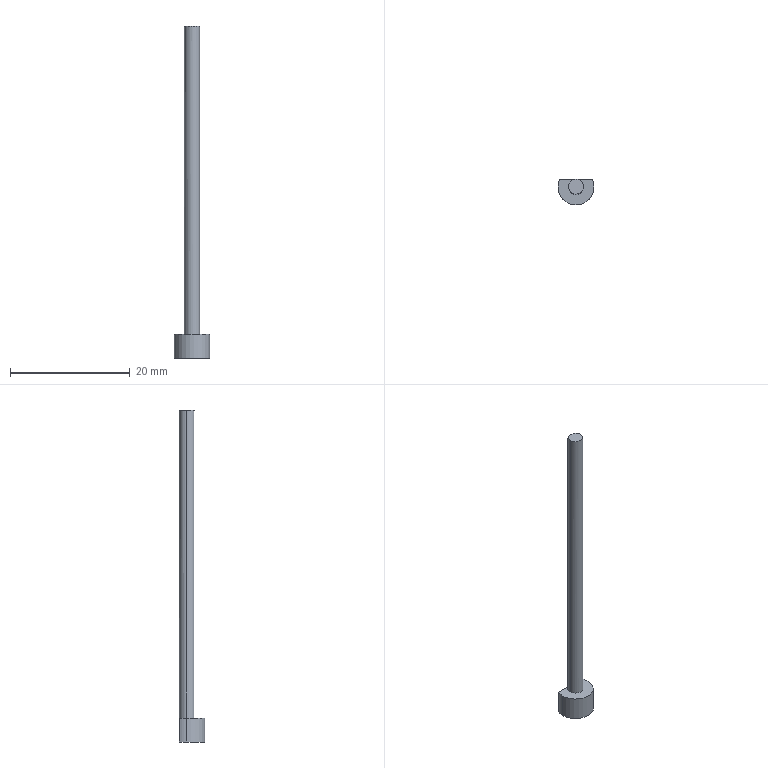Part | STEP file | 1 solid | 10 faces | box 6 x 4.256 x 55.458 mm | volume 340.576 mm3 | cylinder 5 | plane 5 | commonest cylinder face diameters 6 x3 2.513 x2
STEP:
#1=CARTESIAN_POINT('',(0.,0.,0.));
#2=DIRECTION('',(0.,0.,1.));
#3=DIRECTION('',(1.,0.,0.));
#4=AXIS2_PLACEMENT_3D('',#1,#2,#3);
#5=CARTESIAN_POINT('',(-20.312,64.873,-51.47));
#6=VERTEX_POINT('',#5);
#7=CARTESIAN_POINT('',(-20.587,63.617,-51.47));
#8=VERTEX_POINT('',#7);
#9=CARTESIAN_POINT('',(-17.587,63.617,-51.47));
#10=DIRECTION('',(0.,0.,1.));
#11=DIRECTION('',(1.,0.,0.));
#12=AXIS2_PLACEMENT_3D('',#9,#10,#11);
#13=CIRCLE('',#12,3.);
#14=CARTESIAN_POINT('',(-17.587,63.617,-51.47));
#15=DIRECTION('',(0.,0.,1.));
#16=DIRECTION('',(1.,0.,0.));
#17=AXIS2_PLACEMENT_3D('',#14,#15,#16);
#18=CYLINDRICAL_SURFACE('',#17,3.);
#19=CARTESIAN_POINT('',(0.,0.));
#20=DIRECTION('',(1.,0.));
#21=VECTOR('',#20,1.);
#22=LINE('',#19,#21);
#23=(GEOMETRIC_REPRESENTATION_CONTEXT(2)PARAMETRIC_REPRESENTATION_CONTEXT()REPRESENTATION_CONTEXT('',''));
#24=DEFINITIONAL_REPRESENTATION('',(#22),#23);
#25=PCURVE('',#18,#24);
#26=CARTESIAN_POINT('',(-42.862,64.,-51.47));
#27=DIRECTION('',(0.,0.,1.));
#28=DIRECTION('',(1.,0.,0.));
#29=AXIS2_PLACEMENT_3D('',#26,#27,#28);
#30=PLANE('',#29);
#31=CARTESIAN_POINT('',(25.275,-0.3835));
#32=DIRECTION('',(1.,0.));
#33=AXIS2_PLACEMENT_2D('',#31,#32);
#34=CIRCLE('',#33,3.);
#35=(GEOMETRIC_REPRESENTATION_CONTEXT(2)PARAMETRIC_REPRESENTATION_CONTEXT()REPRESENTATION_CONTEXT('',''));
#36=DEFINITIONAL_REPRESENTATION('',(#34),#35);
#37=PCURVE('',#30,#36);
#38=SURFACE_CURVE('',#13,(#25,#37),.PCURVE_S1.);
#39=EDGE_CURVE('',#6,#8,#38,.T.);
#40=ORIENTED_EDGE('',*,*,#39,.T.);
#41=CARTESIAN_POINT('',(-20.587,63.617,-47.47));
#42=VERTEX_POINT('',#41);
#43=CARTESIAN_POINT('',(-20.587,63.617,-51.47));
#44=DIRECTION('',(0.,0.,1.));
#45=VECTOR('',#44,1.);
#46=LINE('',#43,#45);
#47=CARTESIAN_POINT('',(3.142,0.));
#48=DIRECTION('',(0.,1.));
#49=VECTOR('',#48,1.);
#50=LINE('',#47,#49);
#51=(GEOMETRIC_REPRESENTATION_CONTEXT(2)PARAMETRIC_REPRESENTATION_CONTEXT()REPRESENTATION_CONTEXT('',''));
#52=DEFINITIONAL_REPRESENTATION('',(#50),#51);
#53=PCURVE('',#18,#52);
#54=CARTESIAN_POINT('',(-17.587,63.617,-51.47));
#55=DIRECTION('',(0.,0.,1.));
#56=DIRECTION('',(1.,0.,0.));
#57=AXIS2_PLACEMENT_3D('',#54,#55,#56);
#58=CYLINDRICAL_SURFACE('',#57,3.);
#59=CARTESIAN_POINT('',(3.142,0.));
#60=DIRECTION('',(0.,1.));
#61=VECTOR('',#60,1.);
#62=LINE('',#59,#61);
#63=(GEOMETRIC_REPRESENTATION_CONTEXT(2)PARAMETRIC_REPRESENTATION_CONTEXT()REPRESENTATION_CONTEXT('',''));
#64=DEFINITIONAL_REPRESENTATION('',(#62),#63);
#65=PCURVE('',#58,#64);
#66=SURFACE_CURVE('',#46,(#53,#65),.PCURVE_S1.);
#67=EDGE_CURVE('',#8,#42,#66,.T.);
#68=ORIENTED_EDGE('',*,*,#67,.T.);
#69=CARTESIAN_POINT('',(-20.312,64.873,-47.47));
#70=VERTEX_POINT('',#69);
#71=CARTESIAN_POINT('',(-17.587,63.617,-47.47));
#72=DIRECTION('',(0.,0.,-1.));
#73=DIRECTION('',(-1.,0.,0.));
#74=AXIS2_PLACEMENT_3D('',#71,#72,#73);
#75=CIRCLE('',#74,3.);
#76=CARTESIAN_POINT('',(3.142,4.));
#77=DIRECTION('',(-1.,0.));
#78=VECTOR('',#77,1.);
#79=LINE('',#76,#78);
#80=(GEOMETRIC_REPRESENTATION_CONTEXT(2)PARAMETRIC_REPRESENTATION_CONTEXT()REPRESENTATION_CONTEXT('',''));
#81=DEFINITIONAL_REPRESENTATION('',(#79),#80);
#82=PCURVE('',#18,#81);
#83=CARTESIAN_POINT('',(-17.587,63.617,-47.47));
#84=DIRECTION('',(0.,0.,1.));
#85=DIRECTION('',(1.,0.,0.));
#86=AXIS2_PLACEMENT_3D('',#83,#84,#85);
#87=PLANE('',#86);
#88=CARTESIAN_POINT('',(-3.,0.));
#89=CARTESIAN_POINT('',(-3.,5.196));
#90=CARTESIAN_POINT('',(1.5,2.598));
#91=CARTESIAN_POINT('',(6.,0.));
#92=CARTESIAN_POINT('',(1.5,-2.598));
#93=CARTESIAN_POINT('',(-3.,-5.196));
#94=CARTESIAN_POINT('',(-3.,0.));
#95=(BOUNDED_CURVE()B_SPLINE_CURVE(2,(#88,#89,#90,#91,#92,#93,#94),.UNSPECIFIED.,.T.,.F.)B_SPLINE_CURVE_WITH_KNOTS((1,2,2,2,2,1),(-2.094,0.,2.094,4.189,6.283,8.378),.UNSPECIFIED.)CURVE()GEOMETRIC_REPRESENTATION_ITEM()RATIONAL_B_SPLINE_CURVE((1.,0.5,1.,0.5,1.,0.5,1.))REPRESENTATION_ITEM(''));
#96=(GEOMETRIC_REPRESENTATION_CONTEXT(2)PARAMETRIC_REPRESENTATION_CONTEXT()REPRESENTATION_CONTEXT('',''));
#97=DEFINITIONAL_REPRESENTATION('',(#95),#96);
#98=PCURVE('',#87,#97);
#99=SURFACE_CURVE('',#75,(#82,#98),.PCURVE_S1.);
#100=EDGE_CURVE('',#42,#70,#99,.T.);
#101=ORIENTED_EDGE('',*,*,#100,.T.);
#102=CARTESIAN_POINT('',(-20.312,64.873,-51.47));
#103=DIRECTION('',(0.,0.,-1.));
#104=VECTOR('',#103,1.);
#105=LINE('',#102,#104);
#106=CARTESIAN_POINT('',(2.71,0.));
#107=DIRECTION('',(0.,-1.));
#108=VECTOR('',#107,1.);
#109=LINE('',#106,#108);
#110=(GEOMETRIC_REPRESENTATION_CONTEXT(2)PARAMETRIC_REPRESENTATION_CONTEXT()REPRESENTATION_CONTEXT('',''));
#111=DEFINITIONAL_REPRESENTATION('',(#109),#110);
#112=PCURVE('',#18,#111);
#113=CARTESIAN_POINT('',(-17.587,64.873,-51.47));
#114=DIRECTION('',(0.,1.,0.));
#115=DIRECTION('',(0.,0.,1.));
#116=AXIS2_PLACEMENT_3D('',#113,#114,#115);
#117=PLANE('',#116);
#118=CARTESIAN_POINT('',(0.,-2.724));
#119=DIRECTION('',(-1.,0.));
#120=VECTOR('',#119,1.);
#121=LINE('',#118,#120);
#122=(GEOMETRIC_REPRESENTATION_CONTEXT(2)PARAMETRIC_REPRESENTATION_CONTEXT()REPRESENTATION_CONTEXT('',''));
#123=DEFINITIONAL_REPRESENTATION('',(#121),#122);
#124=PCURVE('',#117,#123);
#125=SURFACE_CURVE('',#105,(#112,#124),.PCURVE_S1.);
#126=EDGE_CURVE('',#70,#6,#125,.T.);
#127=ORIENTED_EDGE('',*,*,#126,.T.);
#128=EDGE_LOOP('',(#40,#68,#101,#127));
#129=FACE_BOUND('',#128,.T.);
#130=ADVANCED_FACE('',(#129),#18,.T.);
#131=ORIENTED_EDGE('',*,*,#67,.F.);
#132=CARTESIAN_POINT('',(-14.588,63.617,-51.47));
#133=VERTEX_POINT('',#132);
#134=CARTESIAN_POINT('',(-17.587,63.617,-51.47));
#135=DIRECTION('',(0.,0.,1.));
#136=DIRECTION('',(1.,0.,0.));
#137=AXIS2_PLACEMENT_3D('',#134,#135,#136);
#138=CIRCLE('',#137,3.);
#139=CARTESIAN_POINT('',(0.,0.));
#140=DIRECTION('',(1.,0.));
#141=VECTOR('',#140,1.);
#142=LINE('',#139,#141);
#143=(GEOMETRIC_REPRESENTATION_CONTEXT(2)PARAMETRIC_REPRESENTATION_CONTEXT()REPRESENTATION_CONTEXT('',''));
#144=DEFINITIONAL_REPRESENTATION('',(#142),#143);
#145=PCURVE('',#58,#144);
#146=CARTESIAN_POINT('',(25.275,-0.3835));
#147=DIRECTION('',(1.,0.));
#148=AXIS2_PLACEMENT_2D('',#146,#147);
#149=CIRCLE('',#148,3.);
#150=(GEOMETRIC_REPRESENTATION_CONTEXT(2)PARAMETRIC_REPRESENTATION_CONTEXT()REPRESENTATION_CONTEXT('',''));
#151=DEFINITIONAL_REPRESENTATION('',(#149),#150);
#152=PCURVE('',#30,#151);
#153=SURFACE_CURVE('',#138,(#145,#152),.PCURVE_S1.);
#154=EDGE_CURVE('',#8,#133,#153,.T.);
#155=ORIENTED_EDGE('',*,*,#154,.T.);
#156=CARTESIAN_POINT('',(-14.588,63.617,-47.47));
#157=VERTEX_POINT('',#156);
#158=CARTESIAN_POINT('',(-14.588,63.617,-51.47));
#159=DIRECTION('',(0.,0.,1.));
#160=VECTOR('',#159,1.);
#161=LINE('',#158,#160);
#162=CARTESIAN_POINT('',(6.283,0.));
#163=DIRECTION('',(0.,1.));
#164=VECTOR('',#163,1.);
#165=LINE('',#162,#164);
#166=(GEOMETRIC_REPRESENTATION_CONTEXT(2)PARAMETRIC_REPRESENTATION_CONTEXT()REPRESENTATION_CONTEXT('',''));
#167=DEFINITIONAL_REPRESENTATION('',(#165),#166);
#168=PCURVE('',#58,#167);
#169=CARTESIAN_POINT('',(-17.587,63.617,-51.47));
#170=DIRECTION('',(0.,0.,1.));
#171=DIRECTION('',(1.,0.,0.));
#172=AXIS2_PLACEMENT_3D('',#169,#170,#171);
#173=CYLINDRICAL_SURFACE('',#172,3.);
#174=CARTESIAN_POINT('',(0.,0.));
#175=DIRECTION('',(0.,1.));
#176=VECTOR('',#175,1.);
#177=LINE('',#174,#176);
#178=(GEOMETRIC_REPRESENTATION_CONTEXT(2)PARAMETRIC_REPRESENTATION_CONTEXT()REPRESENTATION_CONTEXT('',''));
#179=DEFINITIONAL_REPRESENTATION('',(#177),#178);
#180=PCURVE('',#173,#179);
#181=SURFACE_CURVE('',#161,(#168,#180),.PCURVE_S1.);
#182=EDGE_CURVE('',#133,#157,#181,.T.);
#183=ORIENTED_EDGE('',*,*,#182,.T.);
#184=CARTESIAN_POINT('',(-17.587,63.617,-47.47));
#185=DIRECTION('',(0.,0.,-1.));
#186=DIRECTION('',(-1.,0.,0.));
#187=AXIS2_PLACEMENT_3D('',#184,#185,#186);
#188=CIRCLE('',#187,3.);
#189=CARTESIAN_POINT('',(9.425,4.));
#190=DIRECTION('',(-1.,0.));
#191=VECTOR('',#190,1.);
#192=LINE('',#189,#191);
#193=(GEOMETRIC_REPRESENTATION_CONTEXT(2)PARAMETRIC_REPRESENTATION_CONTEXT()REPRESENTATION_CONTEXT('',''));
#194=DEFINITIONAL_REPRESENTATION('',(#192),#193);
#195=PCURVE('',#58,#194);
#196=CARTESIAN_POINT('',(-3.,0.));
#197=CARTESIAN_POINT('',(-3.,5.196));
#198=CARTESIAN_POINT('',(1.5,2.598));
#199=CARTESIAN_POINT('',(6.,0.));
#200=CARTESIAN_POINT('',(1.5,-2.598));
#201=CARTESIAN_POINT('',(-3.,-5.196));
#202=CARTESIAN_POINT('',(-3.,0.));
#203=(BOUNDED_CURVE()B_SPLINE_CURVE(2,(#196,#197,#198,#199,#200,#201,#202),.UNSPECIFIED.,.T.,.F.)B_SPLINE_CURVE_WITH_KNOTS((1,2,2,2,2,1),(-2.094,0.,2.094,4.189,6.283,8.378),.UNSPECIFIED.)CURVE()GEOMETRIC_REPRESENTATION_ITEM()RATIONAL_B_SPLINE_CURVE((1.,0.5,1.,0.5,1.,0.5,1.))REPRESENTATION_ITEM(''));
#204=(GEOMETRIC_REPRESENTATION_CONTEXT(2)PARAMETRIC_REPRESENTATION_CONTEXT()REPRESENTATION_CONTEXT('',''));
#205=DEFINITIONAL_REPRESENTATION('',(#203),#204);
#206=PCURVE('',#87,#205);
#207=SURFACE_CURVE('',#188,(#195,#206),.PCURVE_S1.);
#208=EDGE_CURVE('',#157,#42,#207,.T.);
#209=ORIENTED_EDGE('',*,*,#208,.T.);
#210=EDGE_LOOP('',(#131,#155,#183,#209));
#211=FACE_BOUND('',#210,.T.);
#212=ADVANCED_FACE('',(#211),#58,.T.);
#213=CARTESIAN_POINT('',(-18.844,63.617,3.922));
#214=VERTEX_POINT('',#213);
#215=CARTESIAN_POINT('',(-16.331,63.617,3.922));
#216=VERTEX_POINT('',#215);
#217=CARTESIAN_POINT('',(-18.844,63.617,3.922));
#218=CARTESIAN_POINT('',(-18.844,66.129,3.791));
#219=CARTESIAN_POINT('',(-16.331,66.129,3.791));
#220=CARTESIAN_POINT('',(-16.331,63.617,3.922));
#221=(BOUNDED_CURVE()B_SPLINE_CURVE(3,(#217,#218,#219,#220),.UNSPECIFIED.,.F.,.F.)B_SPLINE_CURVE_WITH_KNOTS((4,4),(4.712,7.854),.PIECEWISE_BEZIER_KNOTS.)CURVE()GEOMETRIC_REPRESENTATION_ITEM()RATIONAL_B_SPLINE_CURVE((1.,0.3333,0.3333,1.))REPRESENTATION_ITEM(''));
#222=CARTESIAN_POINT('',(-17.587,63.617,7.478));
#223=DIRECTION('',(0.,0.,-1.));
#224=DIRECTION('',(-1.,0.,0.));
#225=AXIS2_PLACEMENT_3D('',#222,#223,#224);
#226=CYLINDRICAL_SURFACE('',#225,1.256);
#227=CARTESIAN_POINT('',(0.,3.556));
#228=CARTESIAN_POINT('',(0.0303,3.558));
#229=CARTESIAN_POINT('',(0.09367,3.562));
#230=CARTESIAN_POINT('',(0.1977,3.569));
#231=CARTESIAN_POINT('',(0.3115,3.576));
#232=CARTESIAN_POINT('',(0.4356,3.584));
#233=CARTESIAN_POINT('',(0.5703,3.591));
#234=CARTESIAN_POINT('',(0.7158,3.599));
#235=CARTESIAN_POINT('',(0.8717,3.606));
#236=CARTESIAN_POINT('',(1.037,3.613));
#237=CARTESIAN_POINT('',(1.21,3.618));
#238=CARTESIAN_POINT('',(1.389,3.621));
#239=CARTESIAN_POINT('',(1.571,3.622));
#240=CARTESIAN_POINT('',(1.753,3.621));
#241=CARTESIAN_POINT('',(1.931,3.618));
#242=CARTESIAN_POINT('',(2.105,3.613));
#243=CARTESIAN_POINT('',(2.27,3.606));
#244=CARTESIAN_POINT('',(2.426,3.599));
#245=CARTESIAN_POINT('',(2.571,3.591));
#246=CARTESIAN_POINT('',(2.706,3.584));
#247=CARTESIAN_POINT('',(2.83,3.576));
#248=CARTESIAN_POINT('',(2.944,3.569));
#249=CARTESIAN_POINT('',(3.048,3.562));
#250=CARTESIAN_POINT('',(3.111,3.558));
#251=CARTESIAN_POINT('',(3.142,3.556));
#252=B_SPLINE_CURVE_WITH_KNOTS('',3,(#227,#228,#229,#230,#231,#232,#233,#234,#235,#236,#237,#238,#239,#240,#241,#242,#243,#244,#245,#246,#247,#248,#249,#250,#251),.UNSPECIFIED.,.F.,.F.,(4,1,1,1,1,1,1,1,1,1,1,1,1,1,1,1,1,1,1,1,1,1,4),(4.712,4.855,4.998,5.141,5.284,5.426,5.569,5.712,5.855,5.998,6.14,6.283,6.426,6.569,6.712,6.854,6.997,7.14,7.283,7.426,7.568,7.711,7.854),.QUASI_UNIFORM_KNOTS.);
#253=(GEOMETRIC_REPRESENTATION_CONTEXT(2)PARAMETRIC_REPRESENTATION_CONTEXT()REPRESENTATION_CONTEXT('',''));
#254=DEFINITIONAL_REPRESENTATION('',(#252),#253);
#255=PCURVE('',#226,#254);
#256=CARTESIAN_POINT('',(-145.725,90.581,2.509));
#257=DIRECTION('',(0.,-0.05234,-0.9986));
#258=DIRECTION('',(0.,0.9986,-0.05234));
#259=AXIS2_PLACEMENT_3D('',#256,#257,#258);
#260=PLANE('',#259);
#261=CARTESIAN_POINT('',(-27.002,126.881));
#262=CARTESIAN_POINT('',(-24.486,126.881));
#263=CARTESIAN_POINT('',(-24.486,129.394));
#264=CARTESIAN_POINT('',(-27.002,129.394));
#265=(BOUNDED_CURVE()B_SPLINE_CURVE(3,(#261,#262,#263,#264),.UNSPECIFIED.,.F.,.F.)B_SPLINE_CURVE_WITH_KNOTS((4,4),(4.712,7.854),.PIECEWISE_BEZIER_KNOTS.)CURVE()GEOMETRIC_REPRESENTATION_ITEM()RATIONAL_B_SPLINE_CURVE((1.,0.3333,0.3333,1.))REPRESENTATION_ITEM(''));
#266=(GEOMETRIC_REPRESENTATION_CONTEXT(2)PARAMETRIC_REPRESENTATION_CONTEXT()REPRESENTATION_CONTEXT('',''));
#267=DEFINITIONAL_REPRESENTATION('',(#265),#266);
#268=PCURVE('',#260,#267);
#269=SURFACE_CURVE('',#221,(#255,#268),.PCURVE_S1.);
#270=EDGE_CURVE('',#214,#216,#269,.T.);
#271=ORIENTED_EDGE('',*,*,#270,.T.);
#272=CARTESIAN_POINT('',(-16.331,63.617,-47.47));
#273=VERTEX_POINT('',#272);
#274=CARTESIAN_POINT('',(-16.331,63.617,7.478));
#275=DIRECTION('',(0.,0.,-1.));
#276=VECTOR('',#275,1.);
#277=LINE('',#274,#276);
#278=CARTESIAN_POINT('',(3.142,0.));
#279=DIRECTION('',(0.,1.));
#280=VECTOR('',#279,1.);
#281=LINE('',#278,#280);
#282=(GEOMETRIC_REPRESENTATION_CONTEXT(2)PARAMETRIC_REPRESENTATION_CONTEXT()REPRESENTATION_CONTEXT('',''));
#283=DEFINITIONAL_REPRESENTATION('',(#281),#282);
#284=PCURVE('',#226,#283);
#285=CARTESIAN_POINT('',(-17.587,63.617,7.478));
#286=DIRECTION('',(0.,0.,-1.));
#287=DIRECTION('',(-1.,0.,0.));
#288=AXIS2_PLACEMENT_3D('',#285,#286,#287);
#289=CYLINDRICAL_SURFACE('',#288,1.256);
#290=CARTESIAN_POINT('',(3.142,0.));
#291=DIRECTION('',(0.,1.));
#292=VECTOR('',#291,1.);
#293=LINE('',#290,#292);
#294=(GEOMETRIC_REPRESENTATION_CONTEXT(2)PARAMETRIC_REPRESENTATION_CONTEXT()REPRESENTATION_CONTEXT('',''));
#295=DEFINITIONAL_REPRESENTATION('',(#293),#294);
#296=PCURVE('',#289,#295);
#297=SURFACE_CURVE('',#277,(#284,#296),.PCURVE_S1.);
#298=EDGE_CURVE('',#216,#273,#297,.T.);
#299=ORIENTED_EDGE('',*,*,#298,.T.);
#300=CARTESIAN_POINT('',(-17.562,64.873,-47.47));
#301=VERTEX_POINT('',#300);
#302=CARTESIAN_POINT('',(-17.587,63.617,-47.47));
#303=DIRECTION('',(0.,0.,1.));
#304=DIRECTION('',(1.,0.,0.));
#305=AXIS2_PLACEMENT_3D('',#302,#303,#304);
#306=CIRCLE('',#305,1.256);
#307=CARTESIAN_POINT('',(3.142,54.948));
#308=DIRECTION('',(-1.,0.));
#309=VECTOR('',#308,1.);
#310=LINE('',#307,#309);
#311=(GEOMETRIC_REPRESENTATION_CONTEXT(2)PARAMETRIC_REPRESENTATION_CONTEXT()REPRESENTATION_CONTEXT('',''));
#312=DEFINITIONAL_REPRESENTATION('',(#310),#311);
#313=PCURVE('',#226,#312);
#314=CARTESIAN_POINT('',(0.,0.));
#315=DIRECTION('',(1.,0.));
#316=AXIS2_PLACEMENT_2D('',#314,#315);
#317=CIRCLE('',#316,1.256);
#318=(GEOMETRIC_REPRESENTATION_CONTEXT(2)PARAMETRIC_REPRESENTATION_CONTEXT()REPRESENTATION_CONTEXT('',''));
#319=DEFINITIONAL_REPRESENTATION('',(#317),#318);
#320=PCURVE('',#87,#319);
#321=SURFACE_CURVE('',#306,(#313,#320),.PCURVE_S1.);
#322=EDGE_CURVE('',#273,#301,#321,.T.);
#323=ORIENTED_EDGE('',*,*,#322,.T.);
#324=CARTESIAN_POINT('',(-17.562,64.873,-51.47));
#325=VERTEX_POINT('',#324);
#326=CARTESIAN_POINT('',(-17.562,64.873,7.478));
#327=DIRECTION('',(0.,0.,-1.));
#328=VECTOR('',#327,1.);
#329=LINE('',#326,#328);
#330=CARTESIAN_POINT('',(1.591,0.));
#331=DIRECTION('',(0.,1.));
#332=VECTOR('',#331,1.);
#333=LINE('',#330,#332);
#334=(GEOMETRIC_REPRESENTATION_CONTEXT(2)PARAMETRIC_REPRESENTATION_CONTEXT()REPRESENTATION_CONTEXT('',''));
#335=DEFINITIONAL_REPRESENTATION('',(#333),#334);
#336=PCURVE('',#226,#335);
#337=CARTESIAN_POINT('',(-17.587,64.873,-51.47));
#338=DIRECTION('',(0.,1.,0.));
#339=DIRECTION('',(0.,0.,1.));
#340=AXIS2_PLACEMENT_3D('',#337,#338,#339);
#341=PLANE('',#340);
#342=CARTESIAN_POINT('',(58.948,0.02506));
#343=DIRECTION('',(-1.,0.));
#344=VECTOR('',#343,1.);
#345=LINE('',#342,#344);
#346=(GEOMETRIC_REPRESENTATION_CONTEXT(2)PARAMETRIC_REPRESENTATION_CONTEXT()REPRESENTATION_CONTEXT('',''));
#347=DEFINITIONAL_REPRESENTATION('',(#345),#346);
#348=PCURVE('',#341,#347);
#349=SURFACE_CURVE('',#329,(#336,#348),.PCURVE_S1.);
#350=EDGE_CURVE('',#301,#325,#349,.T.);
#351=ORIENTED_EDGE('',*,*,#350,.T.);
#352=CARTESIAN_POINT('',(-17.613,64.873,-51.47));
#353=VERTEX_POINT('',#352);
#354=CARTESIAN_POINT('',(-17.587,63.617,-51.47));
#355=DIRECTION('',(0.,0.,1.));
#356=DIRECTION('',(-1.,0.,0.));
#357=AXIS2_PLACEMENT_3D('',#354,#355,#356);
#358=CIRCLE('',#357,1.256);
#359=CARTESIAN_POINT('',(6.283,58.948));
#360=DIRECTION('',(-1.,0.));
#361=VECTOR('',#360,1.);
#362=LINE('',#359,#361);
#363=(GEOMETRIC_REPRESENTATION_CONTEXT(2)PARAMETRIC_REPRESENTATION_CONTEXT()REPRESENTATION_CONTEXT('',''));
#364=DEFINITIONAL_REPRESENTATION('',(#362),#363);
#365=PCURVE('',#226,#364);
#366=CARTESIAN_POINT('',(25.275,-0.3835));
#367=DIRECTION('',(-1.,0.));
#368=AXIS2_PLACEMENT_2D('',#366,#367);
#369=CIRCLE('',#368,1.256);
#370=(GEOMETRIC_REPRESENTATION_CONTEXT(2)PARAMETRIC_REPRESENTATION_CONTEXT()REPRESENTATION_CONTEXT('',''));
#371=DEFINITIONAL_REPRESENTATION('',(#369),#370);
#372=PCURVE('',#30,#371);
#373=SURFACE_CURVE('',#358,(#365,#372),.PCURVE_S1.);
#374=EDGE_CURVE('',#325,#353,#373,.T.);
#375=ORIENTED_EDGE('',*,*,#374,.T.);
#376=CARTESIAN_POINT('',(-17.613,64.873,-47.47));
#377=VERTEX_POINT('',#376);
#378=CARTESIAN_POINT('',(-17.613,64.873,7.478));
#379=DIRECTION('',(0.,0.,1.));
#380=VECTOR('',#379,1.);
#381=LINE('',#378,#380);
#382=CARTESIAN_POINT('',(1.551,0.));
#383=DIRECTION('',(0.,-1.));
#384=VECTOR('',#383,1.);
#385=LINE('',#382,#384);
#386=(GEOMETRIC_REPRESENTATION_CONTEXT(2)PARAMETRIC_REPRESENTATION_CONTEXT()REPRESENTATION_CONTEXT('',''));
#387=DEFINITIONAL_REPRESENTATION('',(#385),#386);
#388=PCURVE('',#226,#387);
#389=CARTESIAN_POINT('',(58.948,-0.02506));
#390=DIRECTION('',(1.,0.));
#391=VECTOR('',#390,1.);
#392=LINE('',#389,#391);
#393=(GEOMETRIC_REPRESENTATION_CONTEXT(2)PARAMETRIC_REPRESENTATION_CONTEXT()REPRESENTATION_CONTEXT('',''));
#394=DEFINITIONAL_REPRESENTATION('',(#392),#393);
#395=PCURVE('',#117,#394);
#396=SURFACE_CURVE('',#381,(#388,#395),.PCURVE_S1.);
#397=EDGE_CURVE('',#353,#377,#396,.T.);
#398=ORIENTED_EDGE('',*,*,#397,.T.);
#399=CARTESIAN_POINT('',(-18.844,63.617,-47.47));
#400=VERTEX_POINT('',#399);
#401=CARTESIAN_POINT('',(-17.587,63.617,-47.47));
#402=DIRECTION('',(0.,0.,1.));
#403=DIRECTION('',(1.,0.,0.));
#404=AXIS2_PLACEMENT_3D('',#401,#402,#403);
#405=CIRCLE('',#404,1.256);
#406=CARTESIAN_POINT('',(3.142,54.948));
#407=DIRECTION('',(-1.,0.));
#408=VECTOR('',#407,1.);
#409=LINE('',#406,#408);
#410=(GEOMETRIC_REPRESENTATION_CONTEXT(2)PARAMETRIC_REPRESENTATION_CONTEXT()REPRESENTATION_CONTEXT('',''));
#411=DEFINITIONAL_REPRESENTATION('',(#409),#410);
#412=PCURVE('',#226,#411);
#413=CARTESIAN_POINT('',(0.,0.));
#414=DIRECTION('',(1.,0.));
#415=AXIS2_PLACEMENT_2D('',#413,#414);
#416=CIRCLE('',#415,1.256);
#417=(GEOMETRIC_REPRESENTATION_CONTEXT(2)PARAMETRIC_REPRESENTATION_CONTEXT()REPRESENTATION_CONTEXT('',''));
#418=DEFINITIONAL_REPRESENTATION('',(#416),#417);
#419=PCURVE('',#87,#418);
#420=SURFACE_CURVE('',#405,(#412,#419),.PCURVE_S1.);
#421=EDGE_CURVE('',#377,#400,#420,.T.);
#422=ORIENTED_EDGE('',*,*,#421,.T.);
#423=CARTESIAN_POINT('',(-18.844,63.617,7.478));
#424=DIRECTION('',(0.,0.,-1.));
#425=VECTOR('',#424,1.);
#426=LINE('',#423,#425);
#427=CARTESIAN_POINT('',(0.,0.));
#428=DIRECTION('',(0.,1.));
#429=VECTOR('',#428,1.);
#430=LINE('',#427,#429);
#431=(GEOMETRIC_REPRESENTATION_CONTEXT(2)PARAMETRIC_REPRESENTATION_CONTEXT()REPRESENTATION_CONTEXT('',''));
#432=DEFINITIONAL_REPRESENTATION('',(#430),#431);
#433=PCURVE('',#226,#432);
#434=CARTESIAN_POINT('',(6.283,0.));
#435=DIRECTION('',(0.,1.));
#436=VECTOR('',#435,1.);
#437=LINE('',#434,#436);
#438=(GEOMETRIC_REPRESENTATION_CONTEXT(2)PARAMETRIC_REPRESENTATION_CONTEXT()REPRESENTATION_CONTEXT('',''));
#439=DEFINITIONAL_REPRESENTATION('',(#437),#438);
#440=PCURVE('',#289,#439);
#441=SURFACE_CURVE('',#426,(#433,#440),.PCURVE_S1.);
#442=EDGE_CURVE('',#214,#400,#441,.T.);
#443=ORIENTED_EDGE('',*,*,#442,.F.);
#444=EDGE_LOOP('',(#271,#299,#323,#351,#375,#398,#422,#443));
#445=FACE_BOUND('',#444,.T.);
#446=ADVANCED_FACE('',(#445),#226,.T.);
#447=ORIENTED_EDGE('',*,*,#374,.F.);
#448=CARTESIAN_POINT('',(-14.863,64.873,-51.47));
#449=VERTEX_POINT('',#448);
#450=CARTESIAN_POINT('',(-17.587,64.873,-51.47));
#451=DIRECTION('',(1.,0.,0.));
#452=VECTOR('',#451,1.);
#453=LINE('',#450,#452);
#454=CARTESIAN_POINT('',(25.275,0.8725));
#455=DIRECTION('',(1.,0.));
#456=VECTOR('',#455,1.);
#457=LINE('',#454,#456);
#458=(GEOMETRIC_REPRESENTATION_CONTEXT(2)PARAMETRIC_REPRESENTATION_CONTEXT()REPRESENTATION_CONTEXT('',''));
#459=DEFINITIONAL_REPRESENTATION('',(#457),#458);
#460=PCURVE('',#30,#459);
#461=CARTESIAN_POINT('',(0.,0.));
#462=DIRECTION('',(0.,1.));
#463=VECTOR('',#462,1.);
#464=LINE('',#461,#463);
#465=(GEOMETRIC_REPRESENTATION_CONTEXT(2)PARAMETRIC_REPRESENTATION_CONTEXT()REPRESENTATION_CONTEXT('',''));
#466=DEFINITIONAL_REPRESENTATION('',(#464),#465);
#467=PCURVE('',#341,#466);
#468=SURFACE_CURVE('',#453,(#460,#467),.PCURVE_S1.);
#469=EDGE_CURVE('',#325,#449,#468,.T.);
#470=ORIENTED_EDGE('',*,*,#469,.T.);
#471=CARTESIAN_POINT('',(-17.587,63.617,-51.47));
#472=DIRECTION('',(0.,0.,1.));
#473=DIRECTION('',(1.,0.,0.));
#474=AXIS2_PLACEMENT_3D('',#471,#472,#473);
#475=CIRCLE('',#474,3.);
#476=CARTESIAN_POINT('',(25.275,-0.3835));
#477=DIRECTION('',(1.,0.));
#478=AXIS2_PLACEMENT_2D('',#476,#477);
#479=CIRCLE('',#478,3.);
#480=(GEOMETRIC_REPRESENTATION_CONTEXT(2)PARAMETRIC_REPRESENTATION_CONTEXT()REPRESENTATION_CONTEXT('',''));
#481=DEFINITIONAL_REPRESENTATION('',(#479),#480);
#482=PCURVE('',#30,#481);
#483=CARTESIAN_POINT('',(0.,0.));
#484=DIRECTION('',(1.,0.));
#485=VECTOR('',#484,1.);
#486=LINE('',#483,#485);
#487=(GEOMETRIC_REPRESENTATION_CONTEXT(2)PARAMETRIC_REPRESENTATION_CONTEXT()REPRESENTATION_CONTEXT('',''));
#488=DEFINITIONAL_REPRESENTATION('',(#486),#487);
#489=PCURVE('',#173,#488);
#490=SURFACE_CURVE('',#475,(#482,#489),.PCURVE_S1.);
#491=EDGE_CURVE('',#133,#449,#490,.T.);
#492=ORIENTED_EDGE('',*,*,#491,.F.);
#493=ORIENTED_EDGE('',*,*,#154,.F.);
#494=ORIENTED_EDGE('',*,*,#39,.F.);
#495=CARTESIAN_POINT('',(-17.587,64.873,-51.47));
#496=DIRECTION('',(1.,0.,0.));
#497=VECTOR('',#496,1.);
#498=LINE('',#495,#497);
#499=CARTESIAN_POINT('',(25.275,0.8725));
#500=DIRECTION('',(1.,0.));
#501=VECTOR('',#500,1.);
#502=LINE('',#499,#501);
#503=(GEOMETRIC_REPRESENTATION_CONTEXT(2)PARAMETRIC_REPRESENTATION_CONTEXT()REPRESENTATION_CONTEXT('',''));
#504=DEFINITIONAL_REPRESENTATION('',(#502),#503);
#505=PCURVE('',#30,#504);
#506=CARTESIAN_POINT('',(0.,0.));
#507=DIRECTION('',(0.,1.));
#508=VECTOR('',#507,1.);
#509=LINE('',#506,#508);
#510=(GEOMETRIC_REPRESENTATION_CONTEXT(2)PARAMETRIC_REPRESENTATION_CONTEXT()REPRESENTATION_CONTEXT('',''));
#511=DEFINITIONAL_REPRESENTATION('',(#509),#510);
#512=PCURVE('',#117,#511);
#513=SURFACE_CURVE('',#498,(#505,#512),.PCURVE_S1.);
#514=EDGE_CURVE('',#6,#353,#513,.T.);
#515=ORIENTED_EDGE('',*,*,#514,.T.);
#516=EDGE_LOOP('',(#447,#470,#492,#493,#494,#515));
#517=FACE_BOUND('',#516,.T.);
#518=ADVANCED_FACE('',(#517),#30,.F.);
#519=ORIENTED_EDGE('',*,*,#298,.F.);
#520=CARTESIAN_POINT('',(-16.331,63.617,3.922));
#521=CARTESIAN_POINT('',(-16.331,61.104,4.054));
#522=CARTESIAN_POINT('',(-18.844,61.104,4.054));
#523=CARTESIAN_POINT('',(-18.844,63.617,3.922));
#524=(BOUNDED_CURVE()B_SPLINE_CURVE(3,(#520,#521,#522,#523),.UNSPECIFIED.,.F.,.F.)B_SPLINE_CURVE_WITH_KNOTS((4,4),(1.571,4.712),.PIECEWISE_BEZIER_KNOTS.)CURVE()GEOMETRIC_REPRESENTATION_ITEM()RATIONAL_B_SPLINE_CURVE((1.,0.3333,0.3333,1.))REPRESENTATION_ITEM(''));
#525=CARTESIAN_POINT('',(3.142,3.556));
#526=CARTESIAN_POINT('',(3.172,3.554));
#527=CARTESIAN_POINT('',(3.235,3.549));
#528=CARTESIAN_POINT('',(3.339,3.543));
#529=CARTESIAN_POINT('',(3.453,3.535));
#530=CARTESIAN_POINT('',(3.577,3.528));
#531=CARTESIAN_POINT('',(3.712,3.52));
#532=CARTESIAN_POINT('',(3.857,3.512));
#533=CARTESIAN_POINT('',(4.013,3.505));
#534=CARTESIAN_POINT('',(4.179,3.499));
#535=CARTESIAN_POINT('',(4.352,3.494));
#536=CARTESIAN_POINT('',(4.531,3.491));
#537=CARTESIAN_POINT('',(4.712,3.489));
#538=CARTESIAN_POINT('',(4.894,3.491));
#539=CARTESIAN_POINT('',(5.073,3.494));
#540=CARTESIAN_POINT('',(5.246,3.499));
#541=CARTESIAN_POINT('',(5.412,3.505));
#542=CARTESIAN_POINT('',(5.567,3.512));
#543=CARTESIAN_POINT('',(5.713,3.52));
#544=CARTESIAN_POINT('',(5.848,3.528));
#545=CARTESIAN_POINT('',(5.972,3.535));
#546=CARTESIAN_POINT('',(6.085,3.543));
#547=CARTESIAN_POINT('',(6.19,3.549));
#548=CARTESIAN_POINT('',(6.253,3.554));
#549=CARTESIAN_POINT('',(6.283,3.556));
#550=B_SPLINE_CURVE_WITH_KNOTS('',3,(#525,#526,#527,#528,#529,#530,#531,#532,#533,#534,#535,#536,#537,#538,#539,#540,#541,#542,#543,#544,#545,#546,#547,#548,#549),.UNSPECIFIED.,.F.,.F.,(4,1,1,1,1,1,1,1,1,1,1,1,1,1,1,1,1,1,1,1,1,1,4),(1.571,1.714,1.856,1.999,2.142,2.285,2.428,2.57,2.713,2.856,2.999,3.142,3.284,3.427,3.57,3.713,3.856,3.998,4.141,4.284,4.427,4.57,4.712),.QUASI_UNIFORM_KNOTS.);
#551=(GEOMETRIC_REPRESENTATION_CONTEXT(2)PARAMETRIC_REPRESENTATION_CONTEXT()REPRESENTATION_CONTEXT('',''));
#552=DEFINITIONAL_REPRESENTATION('',(#550),#551);
#553=PCURVE('',#289,#552);
#554=CARTESIAN_POINT('',(-27.002,129.394));
#555=CARTESIAN_POINT('',(-29.518,129.394));
#556=CARTESIAN_POINT('',(-29.518,126.881));
#557=CARTESIAN_POINT('',(-27.002,126.881));
#558=(BOUNDED_CURVE()B_SPLINE_CURVE(3,(#554,#555,#556,#557),.UNSPECIFIED.,.F.,.F.)B_SPLINE_CURVE_WITH_KNOTS((4,4),(1.571,4.712),.PIECEWISE_BEZIER_KNOTS.)CURVE()GEOMETRIC_REPRESENTATION_ITEM()RATIONAL_B_SPLINE_CURVE((1.,0.3333,0.3333,1.))REPRESENTATION_ITEM(''));
#559=(GEOMETRIC_REPRESENTATION_CONTEXT(2)PARAMETRIC_REPRESENTATION_CONTEXT()REPRESENTATION_CONTEXT('',''));
#560=DEFINITIONAL_REPRESENTATION('',(#558),#559);
#561=PCURVE('',#260,#560);
#562=SURFACE_CURVE('',#524,(#553,#561),.PCURVE_S1.);
#563=EDGE_CURVE('',#216,#214,#562,.T.);
#564=ORIENTED_EDGE('',*,*,#563,.T.);
#565=ORIENTED_EDGE('',*,*,#442,.T.);
#566=CARTESIAN_POINT('',(-17.587,63.617,-47.47));
#567=DIRECTION('',(0.,0.,1.));
#568=DIRECTION('',(1.,0.,0.));
#569=AXIS2_PLACEMENT_3D('',#566,#567,#568);
#570=CIRCLE('',#569,1.256);
#571=CARTESIAN_POINT('',(9.425,54.948));
#572=DIRECTION('',(-1.,0.));
#573=VECTOR('',#572,1.);
#574=LINE('',#571,#573);
#575=(GEOMETRIC_REPRESENTATION_CONTEXT(2)PARAMETRIC_REPRESENTATION_CONTEXT()REPRESENTATION_CONTEXT('',''));
#576=DEFINITIONAL_REPRESENTATION('',(#574),#575);
#577=PCURVE('',#289,#576);
#578=CARTESIAN_POINT('',(0.,0.));
#579=DIRECTION('',(1.,0.));
#580=AXIS2_PLACEMENT_2D('',#578,#579);
#581=CIRCLE('',#580,1.256);
#582=(GEOMETRIC_REPRESENTATION_CONTEXT(2)PARAMETRIC_REPRESENTATION_CONTEXT()REPRESENTATION_CONTEXT('',''));
#583=DEFINITIONAL_REPRESENTATION('',(#581),#582);
#584=PCURVE('',#87,#583);
#585=SURFACE_CURVE('',#570,(#577,#584),.PCURVE_S1.);
#586=EDGE_CURVE('',#400,#273,#585,.T.);
#587=ORIENTED_EDGE('',*,*,#586,.T.);
#588=EDGE_LOOP('',(#519,#564,#565,#587));
#589=FACE_BOUND('',#588,.T.);
#590=ADVANCED_FACE('',(#589),#289,.T.);
#591=ORIENTED_EDGE('',*,*,#270,.F.);
#592=ORIENTED_EDGE('',*,*,#563,.F.);
#593=EDGE_LOOP('',(#591,#592));
#594=FACE_BOUND('',#593,.T.);
#595=ADVANCED_FACE('',(#594),#260,.F.);
#596=ORIENTED_EDGE('',*,*,#350,.F.);
#597=CARTESIAN_POINT('',(-14.863,64.873,-47.47));
#598=VERTEX_POINT('',#597);
#599=CARTESIAN_POINT('',(-17.587,64.873,-47.47));
#600=DIRECTION('',(-1.,0.,0.));
#601=VECTOR('',#600,1.);
#602=LINE('',#599,#601);
#603=CARTESIAN_POINT('',(4.,0.));
#604=DIRECTION('',(0.,-1.));
#605=VECTOR('',#604,1.);
#606=LINE('',#603,#605);
#607=(GEOMETRIC_REPRESENTATION_CONTEXT(2)PARAMETRIC_REPRESENTATION_CONTEXT()REPRESENTATION_CONTEXT('',''));
#608=DEFINITIONAL_REPRESENTATION('',(#606),#607);
#609=PCURVE('',#341,#608);
#610=CARTESIAN_POINT('',(0.,1.256));
#611=DIRECTION('',(-1.,0.));
#612=VECTOR('',#611,1.);
#613=LINE('',#610,#612);
#614=(GEOMETRIC_REPRESENTATION_CONTEXT(2)PARAMETRIC_REPRESENTATION_CONTEXT()REPRESENTATION_CONTEXT('',''));
#615=DEFINITIONAL_REPRESENTATION('',(#613),#614);
#616=PCURVE('',#87,#615);
#617=SURFACE_CURVE('',#602,(#609,#616),.PCURVE_S1.);
#618=EDGE_CURVE('',#598,#301,#617,.T.);
#619=ORIENTED_EDGE('',*,*,#618,.F.);
#620=CARTESIAN_POINT('',(-14.863,64.873,-51.47));
#621=DIRECTION('',(0.,0.,1.));
#622=VECTOR('',#621,1.);
#623=LINE('',#620,#622);
#624=CARTESIAN_POINT('',(0.,2.724));
#625=DIRECTION('',(1.,0.));
#626=VECTOR('',#625,1.);
#627=LINE('',#624,#626);
#628=(GEOMETRIC_REPRESENTATION_CONTEXT(2)PARAMETRIC_REPRESENTATION_CONTEXT()REPRESENTATION_CONTEXT('',''));
#629=DEFINITIONAL_REPRESENTATION('',(#627),#628);
#630=PCURVE('',#341,#629);
#631=CARTESIAN_POINT('',(0.432,0.));
#632=DIRECTION('',(0.,1.));
#633=VECTOR('',#632,1.);
#634=LINE('',#631,#633);
#635=(GEOMETRIC_REPRESENTATION_CONTEXT(2)PARAMETRIC_REPRESENTATION_CONTEXT()REPRESENTATION_CONTEXT('',''));
#636=DEFINITIONAL_REPRESENTATION('',(#634),#635);
#637=PCURVE('',#173,#636);
#638=SURFACE_CURVE('',#623,(#630,#637),.PCURVE_S1.);
#639=EDGE_CURVE('',#449,#598,#638,.T.);
#640=ORIENTED_EDGE('',*,*,#639,.F.);
#641=ORIENTED_EDGE('',*,*,#469,.F.);
#642=EDGE_LOOP('',(#596,#619,#640,#641));
#643=FACE_BOUND('',#642,.T.);
#644=ADVANCED_FACE('',(#643),#341,.T.);
#645=ORIENTED_EDGE('',*,*,#397,.F.);
#646=ORIENTED_EDGE('',*,*,#514,.F.);
#647=ORIENTED_EDGE('',*,*,#126,.F.);
#648=CARTESIAN_POINT('',(-17.587,64.873,-47.47));
#649=DIRECTION('',(-1.,0.,0.));
#650=VECTOR('',#649,1.);
#651=LINE('',#648,#650);
#652=CARTESIAN_POINT('',(4.,0.));
#653=DIRECTION('',(0.,-1.));
#654=VECTOR('',#653,1.);
#655=LINE('',#652,#654);
#656=(GEOMETRIC_REPRESENTATION_CONTEXT(2)PARAMETRIC_REPRESENTATION_CONTEXT()REPRESENTATION_CONTEXT('',''));
#657=DEFINITIONAL_REPRESENTATION('',(#655),#656);
#658=PCURVE('',#117,#657);
#659=CARTESIAN_POINT('',(0.,1.256));
#660=DIRECTION('',(-1.,0.));
#661=VECTOR('',#660,1.);
#662=LINE('',#659,#661);
#663=(GEOMETRIC_REPRESENTATION_CONTEXT(2)PARAMETRIC_REPRESENTATION_CONTEXT()REPRESENTATION_CONTEXT('',''));
#664=DEFINITIONAL_REPRESENTATION('',(#662),#663);
#665=PCURVE('',#87,#664);
#666=SURFACE_CURVE('',#651,(#658,#665),.PCURVE_S1.);
#667=EDGE_CURVE('',#377,#70,#666,.T.);
#668=ORIENTED_EDGE('',*,*,#667,.F.);
#669=EDGE_LOOP('',(#645,#646,#647,#668));
#670=FACE_BOUND('',#669,.T.);
#671=ADVANCED_FACE('',(#670),#117,.T.);
#672=ORIENTED_EDGE('',*,*,#421,.F.);
#673=ORIENTED_EDGE('',*,*,#667,.T.);
#674=ORIENTED_EDGE('',*,*,#100,.F.);
#675=ORIENTED_EDGE('',*,*,#208,.F.);
#676=CARTESIAN_POINT('',(-17.587,63.617,-47.47));
#677=DIRECTION('',(0.,0.,-1.));
#678=DIRECTION('',(-1.,0.,0.));
#679=AXIS2_PLACEMENT_3D('',#676,#677,#678);
#680=CIRCLE('',#679,3.);
#681=CARTESIAN_POINT('',(-3.,0.));
#682=CARTESIAN_POINT('',(-3.,5.196));
#683=CARTESIAN_POINT('',(1.5,2.598));
#684=CARTESIAN_POINT('',(6.,0.));
#685=CARTESIAN_POINT('',(1.5,-2.598));
#686=CARTESIAN_POINT('',(-3.,-5.196));
#687=CARTESIAN_POINT('',(-3.,0.));
#688=(BOUNDED_CURVE()B_SPLINE_CURVE(2,(#681,#682,#683,#684,#685,#686,#687),.UNSPECIFIED.,.T.,.F.)B_SPLINE_CURVE_WITH_KNOTS((1,2,2,2,2,1),(-2.094,0.,2.094,4.189,6.283,8.378),.UNSPECIFIED.)CURVE()GEOMETRIC_REPRESENTATION_ITEM()RATIONAL_B_SPLINE_CURVE((1.,0.5,1.,0.5,1.,0.5,1.))REPRESENTATION_ITEM(''));
#689=(GEOMETRIC_REPRESENTATION_CONTEXT(2)PARAMETRIC_REPRESENTATION_CONTEXT()REPRESENTATION_CONTEXT('',''));
#690=DEFINITIONAL_REPRESENTATION('',(#688),#689);
#691=PCURVE('',#87,#690);
#692=CARTESIAN_POINT('',(3.142,4.));
#693=DIRECTION('',(-1.,0.));
#694=VECTOR('',#693,1.);
#695=LINE('',#692,#694);
#696=(GEOMETRIC_REPRESENTATION_CONTEXT(2)PARAMETRIC_REPRESENTATION_CONTEXT()REPRESENTATION_CONTEXT('',''));
#697=DEFINITIONAL_REPRESENTATION('',(#695),#696);
#698=PCURVE('',#173,#697);
#699=SURFACE_CURVE('',#680,(#691,#698),.PCURVE_S1.);
#700=EDGE_CURVE('',#598,#157,#699,.T.);
#701=ORIENTED_EDGE('',*,*,#700,.F.);
#702=ORIENTED_EDGE('',*,*,#618,.T.);
#703=ORIENTED_EDGE('',*,*,#322,.F.);
#704=ORIENTED_EDGE('',*,*,#586,.F.);
#705=EDGE_LOOP('',(#672,#673,#674,#675,#701,#702,#703,#704));
#706=FACE_BOUND('',#705,.T.);
#707=ADVANCED_FACE('',(#706),#87,.T.);
#708=ORIENTED_EDGE('',*,*,#182,.F.);
#709=ORIENTED_EDGE('',*,*,#491,.T.);
#710=ORIENTED_EDGE('',*,*,#639,.T.);
#711=ORIENTED_EDGE('',*,*,#700,.T.);
#712=EDGE_LOOP('',(#708,#709,#710,#711));
#713=FACE_BOUND('',#712,.T.);
#714=ADVANCED_FACE('',(#713),#173,.T.);
#715=CLOSED_SHELL('',(#130,#212,#446,#518,#590,#595,#644,#671,#707,#714));
#716=MANIFOLD_SOLID_BREP('',#715);
#717=(LENGTH_UNIT()NAMED_UNIT(*)SI_UNIT(.MILLI.,.METRE.));
#718=UNCERTAINTY_MEASURE_WITH_UNIT(LENGTH_MEASURE(0.0000001),#717,'','');
#719=(NAMED_UNIT(*)PLANE_ANGLE_UNIT()SI_UNIT($,.RADIAN.));
#720=(NAMED_UNIT(*)SI_UNIT($,.STERADIAN.)SOLID_ANGLE_UNIT());
#721=(GEOMETRIC_REPRESENTATION_CONTEXT(3)GLOBAL_UNCERTAINTY_ASSIGNED_CONTEXT((#718))GLOBAL_UNIT_ASSIGNED_CONTEXT((#717,#719,#720))REPRESENTATION_CONTEXT('',''));
#722=ADVANCED_BREP_SHAPE_REPRESENTATION('',(#4,#716),#721);